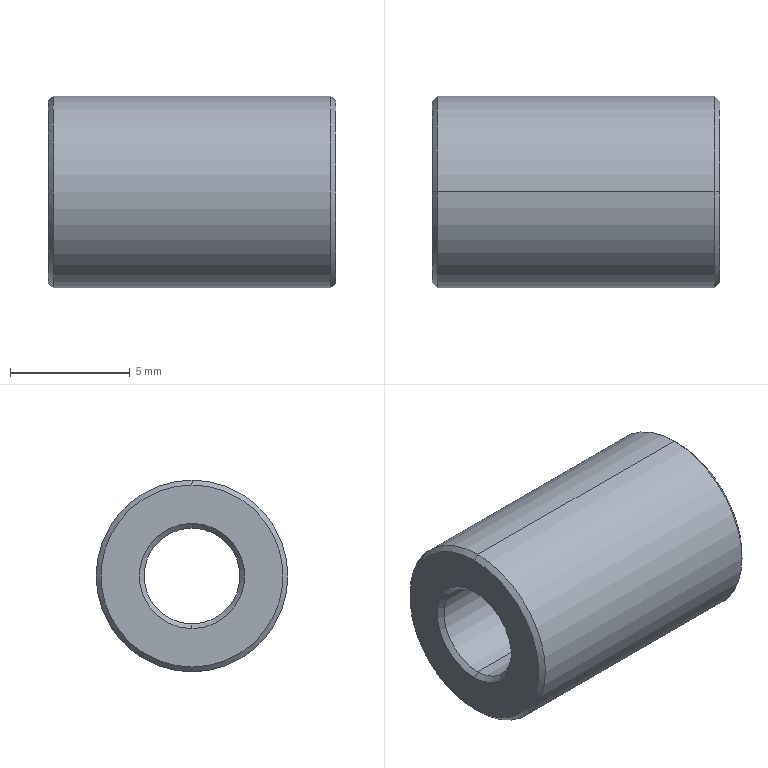Part | SolidWorks | features RefAxis 3, 3DProfileFeature 1, Chamfer 1, Revolution 1 | 1 solid | 14 faces | box 12 x 8 x 8 mm | volume 450.881 mm3 | cone 8 | cylinder 4 | plane 2 | commonest cylinder face diameters 4 x2 8 x2
STEP:
#1=CARTESIAN_POINT('',(0.,0.,3.8));
#2=VERTEX_POINT('',#1);
#3=CARTESIAN_POINT('',(0.,0.,-3.8));
#4=VERTEX_POINT('',#3);
#5=CARTESIAN_POINT('',(0.,0.,0.));
#6=DIRECTION('',(-1.,0.,0.));
#7=DIRECTION('',(0.,0.,-1.));
#8=AXIS2_PLACEMENT_3D('',#5,#6,#7);
#9=CIRCLE('',#8,3.8);
#10=EDGE_CURVE('',#2,#4,#9,.T.);
#11=ORIENTED_EDGE('',*,*,#10,.F.);
#12=CARTESIAN_POINT('',(0.2,0.,4.));
#13=VERTEX_POINT('',#12);
#14=CARTESIAN_POINT('',(0.,0.,3.8));
#15=DIRECTION('',(0.7071,0.,0.7071));
#16=VECTOR('',#15,1000.);
#17=LINE('',#14,#16);
#18=EDGE_CURVE('',#2,#13,#17,.T.);
#19=ORIENTED_EDGE('',*,*,#18,.T.);
#20=CARTESIAN_POINT('',(0.2,0.,-4.));
#21=VERTEX_POINT('',#20);
#22=CARTESIAN_POINT('',(0.2,0.,0.));
#23=DIRECTION('',(1.,0.,0.));
#24=DIRECTION('',(0.,0.,-1.));
#25=AXIS2_PLACEMENT_3D('',#22,#23,#24);
#26=CIRCLE('',#25,4.);
#27=EDGE_CURVE('',#21,#13,#26,.T.);
#28=ORIENTED_EDGE('',*,*,#27,.F.);
#29=CARTESIAN_POINT('',(0.,0.,-3.8));
#30=DIRECTION('',(0.7071,0.,-0.7071));
#31=VECTOR('',#30,1000.);
#32=LINE('',#29,#31);
#33=EDGE_CURVE('',#4,#21,#32,.T.);
#34=ORIENTED_EDGE('',*,*,#33,.F.);
#35=EDGE_LOOP('',(#11,#19,#28,#34));
#36=FACE_OUTER_BOUND('',#35,.T.);
#37=CARTESIAN_POINT('',(0.,0.,0.));
#38=DIRECTION('',(1.,0.,0.));
#39=DIRECTION('',(0.,0.,-1.));
#40=AXIS2_PLACEMENT_3D('',#37,#38,#39);
#41=CONICAL_SURFACE('',#40,3.8,0.7854);
#42=ADVANCED_FACE('',(#36),#41,.T.);
#43=CARTESIAN_POINT('',(12.,0.,-3.8));
#44=VERTEX_POINT('',#43);
#45=CARTESIAN_POINT('',(12.,0.,3.8));
#46=VERTEX_POINT('',#45);
#47=CARTESIAN_POINT('',(12.,0.,0.));
#48=DIRECTION('',(1.,0.,0.));
#49=DIRECTION('',(0.,0.,1.));
#50=AXIS2_PLACEMENT_3D('',#47,#48,#49);
#51=CIRCLE('',#50,3.8);
#52=EDGE_CURVE('',#44,#46,#51,.T.);
#53=ORIENTED_EDGE('',*,*,#52,.F.);
#54=CARTESIAN_POINT('',(11.8,0.,-4.));
#55=VERTEX_POINT('',#54);
#56=CARTESIAN_POINT('',(11.8,0.,-4.));
#57=DIRECTION('',(-0.7071,0.,-0.7071));
#58=VECTOR('',#57,1000.);
#59=LINE('',#56,#58);
#60=EDGE_CURVE('',#44,#55,#59,.T.);
#61=ORIENTED_EDGE('',*,*,#60,.T.);
#62=CARTESIAN_POINT('',(11.8,0.,4.));
#63=VERTEX_POINT('',#62);
#64=CARTESIAN_POINT('',(11.8,0.,0.));
#65=DIRECTION('',(-1.,0.,0.));
#66=DIRECTION('',(0.,0.,1.));
#67=AXIS2_PLACEMENT_3D('',#64,#65,#66);
#68=CIRCLE('',#67,4.);
#69=EDGE_CURVE('',#63,#55,#68,.T.);
#70=ORIENTED_EDGE('',*,*,#69,.F.);
#71=CARTESIAN_POINT('',(11.8,0.,4.));
#72=DIRECTION('',(-0.7071,0.,0.7071));
#73=VECTOR('',#72,1000.);
#74=LINE('',#71,#73);
#75=EDGE_CURVE('',#46,#63,#74,.T.);
#76=ORIENTED_EDGE('',*,*,#75,.F.);
#77=EDGE_LOOP('',(#53,#61,#70,#76));
#78=FACE_OUTER_BOUND('',#77,.T.);
#79=CARTESIAN_POINT('',(11.8,0.,0.));
#80=DIRECTION('',(-1.,0.,0.));
#81=DIRECTION('',(0.,0.,1.));
#82=AXIS2_PLACEMENT_3D('',#79,#80,#81);
#83=CONICAL_SURFACE('',#82,4.,0.7854);
#84=ADVANCED_FACE('',(#78),#83,.T.);
#85=CARTESIAN_POINT('',(0.2,0.,-2.));
#86=VERTEX_POINT('',#85);
#87=CARTESIAN_POINT('',(0.2,0.,2.));
#88=VERTEX_POINT('',#87);
#89=CARTESIAN_POINT('',(0.2,0.,0.));
#90=DIRECTION('',(-1.,0.,0.));
#91=DIRECTION('',(0.,0.,-1.));
#92=AXIS2_PLACEMENT_3D('',#89,#90,#91);
#93=CIRCLE('',#92,2.);
#94=EDGE_CURVE('',#86,#88,#93,.T.);
#95=ORIENTED_EDGE('',*,*,#94,.F.);
#96=CARTESIAN_POINT('',(0.,0.,-2.2));
#97=VERTEX_POINT('',#96);
#98=CARTESIAN_POINT('',(0.2,0.,-2.));
#99=DIRECTION('',(-0.7071,0.,-0.7071));
#100=VECTOR('',#99,1000.);
#101=LINE('',#98,#100);
#102=EDGE_CURVE('',#86,#97,#101,.T.);
#103=ORIENTED_EDGE('',*,*,#102,.T.);
#104=CARTESIAN_POINT('',(0.,0.,2.2));
#105=VERTEX_POINT('',#104);
#106=CARTESIAN_POINT('',(0.,0.,0.));
#107=DIRECTION('',(1.,0.,0.));
#108=DIRECTION('',(0.,0.,-1.));
#109=AXIS2_PLACEMENT_3D('',#106,#107,#108);
#110=CIRCLE('',#109,2.2);
#111=EDGE_CURVE('',#105,#97,#110,.T.);
#112=ORIENTED_EDGE('',*,*,#111,.F.);
#113=CARTESIAN_POINT('',(0.2,0.,2.));
#114=DIRECTION('',(-0.7071,0.,0.7071));
#115=VECTOR('',#114,1000.);
#116=LINE('',#113,#115);
#117=EDGE_CURVE('',#88,#105,#116,.T.);
#118=ORIENTED_EDGE('',*,*,#117,.F.);
#119=EDGE_LOOP('',(#95,#103,#112,#118));
#120=FACE_OUTER_BOUND('',#119,.T.);
#121=CARTESIAN_POINT('',(0.2,0.,0.));
#122=DIRECTION('',(-1.,0.,0.));
#123=DIRECTION('',(0.,0.,1.));
#124=AXIS2_PLACEMENT_3D('',#121,#122,#123);
#125=CONICAL_SURFACE('',#124,2.,0.7854);
#126=ADVANCED_FACE('',(#120),#125,.F.);
#127=CARTESIAN_POINT('',(11.8,0.,2.));
#128=VERTEX_POINT('',#127);
#129=CARTESIAN_POINT('',(11.8,0.,-2.));
#130=VERTEX_POINT('',#129);
#131=CARTESIAN_POINT('',(11.8,0.,0.));
#132=DIRECTION('',(1.,0.,0.));
#133=DIRECTION('',(0.,0.,1.));
#134=AXIS2_PLACEMENT_3D('',#131,#132,#133);
#135=CIRCLE('',#134,2.);
#136=EDGE_CURVE('',#128,#130,#135,.T.);
#137=ORIENTED_EDGE('',*,*,#136,.F.);
#138=CARTESIAN_POINT('',(12.,0.,2.2));
#139=VERTEX_POINT('',#138);
#140=CARTESIAN_POINT('',(12.,0.,2.2));
#141=DIRECTION('',(0.7071,0.,0.7071));
#142=VECTOR('',#141,1000.);
#143=LINE('',#140,#142);
#144=EDGE_CURVE('',#128,#139,#143,.T.);
#145=ORIENTED_EDGE('',*,*,#144,.T.);
#146=CARTESIAN_POINT('',(12.,0.,-2.2));
#147=VERTEX_POINT('',#146);
#148=CARTESIAN_POINT('',(12.,0.,0.));
#149=DIRECTION('',(-1.,0.,0.));
#150=DIRECTION('',(0.,0.,1.));
#151=AXIS2_PLACEMENT_3D('',#148,#149,#150);
#152=CIRCLE('',#151,2.2);
#153=EDGE_CURVE('',#147,#139,#152,.T.);
#154=ORIENTED_EDGE('',*,*,#153,.F.);
#155=CARTESIAN_POINT('',(12.,0.,-2.2));
#156=DIRECTION('',(0.7071,0.,-0.7071));
#157=VECTOR('',#156,1000.);
#158=LINE('',#155,#157);
#159=EDGE_CURVE('',#130,#147,#158,.T.);
#160=ORIENTED_EDGE('',*,*,#159,.F.);
#161=EDGE_LOOP('',(#137,#145,#154,#160));
#162=FACE_OUTER_BOUND('',#161,.T.);
#163=CARTESIAN_POINT('',(12.,0.,0.));
#164=DIRECTION('',(1.,0.,0.));
#165=DIRECTION('',(0.,0.,-1.));
#166=AXIS2_PLACEMENT_3D('',#163,#164,#165);
#167=CONICAL_SURFACE('',#166,2.2,0.7854);
#168=ADVANCED_FACE('',(#162),#167,.F.);
#169=ORIENTED_EDGE('',*,*,#69,.T.);
#170=CARTESIAN_POINT('',(12.,0.,-4.));
#171=DIRECTION('',(-1.,0.,0.));
#172=VECTOR('',#171,1000.);
#173=LINE('',#170,#172);
#174=EDGE_CURVE('',#55,#21,#173,.T.);
#175=ORIENTED_EDGE('',*,*,#174,.T.);
#176=ORIENTED_EDGE('',*,*,#27,.T.);
#177=CARTESIAN_POINT('',(12.,0.,4.));
#178=DIRECTION('',(-1.,0.,0.));
#179=VECTOR('',#178,1000.);
#180=LINE('',#177,#179);
#181=EDGE_CURVE('',#63,#13,#180,.T.);
#182=ORIENTED_EDGE('',*,*,#181,.F.);
#183=EDGE_LOOP('',(#169,#175,#176,#182));
#184=FACE_OUTER_BOUND('',#183,.T.);
#185=CARTESIAN_POINT('',(12.,0.,0.));
#186=DIRECTION('',(-1.,0.,0.));
#187=DIRECTION('',(0.,0.,1.));
#188=AXIS2_PLACEMENT_3D('',#185,#186,#187);
#189=CYLINDRICAL_SURFACE('',#188,4.);
#190=ADVANCED_FACE('',(#184),#189,.T.);
#191=ORIENTED_EDGE('',*,*,#136,.T.);
#192=CARTESIAN_POINT('',(12.,0.,-2.));
#193=DIRECTION('',(-1.,0.,0.));
#194=VECTOR('',#193,1000.);
#195=LINE('',#192,#194);
#196=EDGE_CURVE('',#130,#86,#195,.T.);
#197=ORIENTED_EDGE('',*,*,#196,.T.);
#198=ORIENTED_EDGE('',*,*,#94,.T.);
#199=CARTESIAN_POINT('',(12.,0.,2.));
#200=DIRECTION('',(-1.,0.,0.));
#201=VECTOR('',#200,1000.);
#202=LINE('',#199,#201);
#203=EDGE_CURVE('',#128,#88,#202,.T.);
#204=ORIENTED_EDGE('',*,*,#203,.F.);
#205=EDGE_LOOP('',(#191,#197,#198,#204));
#206=FACE_OUTER_BOUND('',#205,.T.);
#207=CARTESIAN_POINT('',(12.,0.,0.));
#208=DIRECTION('',(-1.,0.,0.));
#209=DIRECTION('',(0.,0.,1.));
#210=AXIS2_PLACEMENT_3D('',#207,#208,#209);
#211=CYLINDRICAL_SURFACE('',#210,2.);
#212=ADVANCED_FACE('',(#206),#211,.F.);
#213=ORIENTED_EDGE('',*,*,#111,.T.);
#214=CARTESIAN_POINT('',(0.,0.,0.));
#215=DIRECTION('',(1.,0.,0.));
#216=DIRECTION('',(0.,0.,-1.));
#217=AXIS2_PLACEMENT_3D('',#214,#215,#216);
#218=CIRCLE('',#217,2.2);
#219=EDGE_CURVE('',#97,#105,#218,.T.);
#220=ORIENTED_EDGE('',*,*,#219,.T.);
#221=EDGE_LOOP('',(#213,#220));
#222=FACE_BOUND('',#221,.T.);
#223=CARTESIAN_POINT('',(0.,0.,0.));
#224=DIRECTION('',(-1.,0.,0.));
#225=DIRECTION('',(0.,0.,-1.));
#226=AXIS2_PLACEMENT_3D('',#223,#224,#225);
#227=CIRCLE('',#226,3.8);
#228=EDGE_CURVE('',#4,#2,#227,.T.);
#229=ORIENTED_EDGE('',*,*,#228,.T.);
#230=ORIENTED_EDGE('',*,*,#10,.T.);
#231=EDGE_LOOP('',(#229,#230));
#232=FACE_OUTER_BOUND('',#231,.T.);
#233=CARTESIAN_POINT('',(0.,3.7,0.));
#234=DIRECTION('',(1.,0.,0.));
#235=DIRECTION('',(0.,0.,-1.));
#236=AXIS2_PLACEMENT_3D('',#233,#234,#235);
#237=PLANE('',#236);
#238=ADVANCED_FACE('',(#222,#232),#237,.F.);
#239=ORIENTED_EDGE('',*,*,#196,.F.);
#240=CARTESIAN_POINT('',(11.8,0.,0.));
#241=DIRECTION('',(1.,0.,0.));
#242=DIRECTION('',(0.,0.,1.));
#243=AXIS2_PLACEMENT_3D('',#240,#241,#242);
#244=CIRCLE('',#243,2.);
#245=EDGE_CURVE('',#130,#128,#244,.T.);
#246=ORIENTED_EDGE('',*,*,#245,.T.);
#247=ORIENTED_EDGE('',*,*,#203,.T.);
#248=CARTESIAN_POINT('',(0.2,0.,0.));
#249=DIRECTION('',(-1.,0.,0.));
#250=DIRECTION('',(0.,0.,-1.));
#251=AXIS2_PLACEMENT_3D('',#248,#249,#250);
#252=CIRCLE('',#251,2.);
#253=EDGE_CURVE('',#88,#86,#252,.T.);
#254=ORIENTED_EDGE('',*,*,#253,.T.);
#255=EDGE_LOOP('',(#239,#246,#247,#254));
#256=FACE_OUTER_BOUND('',#255,.T.);
#257=CARTESIAN_POINT('',(12.,0.,0.));
#258=DIRECTION('',(-1.,0.,0.));
#259=DIRECTION('',(0.,0.,1.));
#260=AXIS2_PLACEMENT_3D('',#257,#258,#259);
#261=CYLINDRICAL_SURFACE('',#260,2.);
#262=ADVANCED_FACE('',(#256),#261,.F.);
#263=ORIENTED_EDGE('',*,*,#153,.T.);
#264=CARTESIAN_POINT('',(12.,0.,0.));
#265=DIRECTION('',(-1.,0.,0.));
#266=DIRECTION('',(0.,0.,1.));
#267=AXIS2_PLACEMENT_3D('',#264,#265,#266);
#268=CIRCLE('',#267,2.2);
#269=EDGE_CURVE('',#139,#147,#268,.T.);
#270=ORIENTED_EDGE('',*,*,#269,.T.);
#271=EDGE_LOOP('',(#263,#270));
#272=FACE_BOUND('',#271,.T.);
#273=CARTESIAN_POINT('',(12.,0.,0.));
#274=DIRECTION('',(1.,0.,0.));
#275=DIRECTION('',(0.,0.,1.));
#276=AXIS2_PLACEMENT_3D('',#273,#274,#275);
#277=CIRCLE('',#276,3.8);
#278=EDGE_CURVE('',#46,#44,#277,.T.);
#279=ORIENTED_EDGE('',*,*,#278,.T.);
#280=ORIENTED_EDGE('',*,*,#52,.T.);
#281=EDGE_LOOP('',(#279,#280));
#282=FACE_OUTER_BOUND('',#281,.T.);
#283=CARTESIAN_POINT('',(12.,3.7,0.));
#284=DIRECTION('',(-1.,0.,0.));
#285=DIRECTION('',(0.,0.,1.));
#286=AXIS2_PLACEMENT_3D('',#283,#284,#285);
#287=PLANE('',#286);
#288=ADVANCED_FACE('',(#272,#282),#287,.F.);
#289=ORIENTED_EDGE('',*,*,#174,.F.);
#290=CARTESIAN_POINT('',(11.8,0.,0.));
#291=DIRECTION('',(-1.,0.,0.));
#292=DIRECTION('',(0.,0.,1.));
#293=AXIS2_PLACEMENT_3D('',#290,#291,#292);
#294=CIRCLE('',#293,4.);
#295=EDGE_CURVE('',#55,#63,#294,.T.);
#296=ORIENTED_EDGE('',*,*,#295,.T.);
#297=ORIENTED_EDGE('',*,*,#181,.T.);
#298=CARTESIAN_POINT('',(0.2,0.,0.));
#299=DIRECTION('',(1.,0.,0.));
#300=DIRECTION('',(0.,0.,-1.));
#301=AXIS2_PLACEMENT_3D('',#298,#299,#300);
#302=CIRCLE('',#301,4.);
#303=EDGE_CURVE('',#13,#21,#302,.T.);
#304=ORIENTED_EDGE('',*,*,#303,.T.);
#305=EDGE_LOOP('',(#289,#296,#297,#304));
#306=FACE_OUTER_BOUND('',#305,.T.);
#307=CARTESIAN_POINT('',(12.,0.,0.));
#308=DIRECTION('',(-1.,0.,0.));
#309=DIRECTION('',(0.,0.,1.));
#310=AXIS2_PLACEMENT_3D('',#307,#308,#309);
#311=CYLINDRICAL_SURFACE('',#310,4.);
#312=ADVANCED_FACE('',(#306),#311,.T.);
#313=ORIENTED_EDGE('',*,*,#144,.F.);
#314=ORIENTED_EDGE('',*,*,#245,.F.);
#315=ORIENTED_EDGE('',*,*,#159,.T.);
#316=ORIENTED_EDGE('',*,*,#269,.F.);
#317=EDGE_LOOP('',(#313,#314,#315,#316));
#318=FACE_OUTER_BOUND('',#317,.T.);
#319=CARTESIAN_POINT('',(12.,0.,0.));
#320=DIRECTION('',(1.,0.,0.));
#321=DIRECTION('',(0.,0.,-1.));
#322=AXIS2_PLACEMENT_3D('',#319,#320,#321);
#323=CONICAL_SURFACE('',#322,2.2,0.7854);
#324=ADVANCED_FACE('',(#318),#323,.F.);
#325=ORIENTED_EDGE('',*,*,#102,.F.);
#326=ORIENTED_EDGE('',*,*,#253,.F.);
#327=ORIENTED_EDGE('',*,*,#117,.T.);
#328=ORIENTED_EDGE('',*,*,#219,.F.);
#329=EDGE_LOOP('',(#325,#326,#327,#328));
#330=FACE_OUTER_BOUND('',#329,.T.);
#331=CARTESIAN_POINT('',(0.2,0.,0.));
#332=DIRECTION('',(-1.,0.,0.));
#333=DIRECTION('',(0.,0.,1.));
#334=AXIS2_PLACEMENT_3D('',#331,#332,#333);
#335=CONICAL_SURFACE('',#334,2.,0.7854);
#336=ADVANCED_FACE('',(#330),#335,.F.);
#337=ORIENTED_EDGE('',*,*,#60,.F.);
#338=ORIENTED_EDGE('',*,*,#278,.F.);
#339=ORIENTED_EDGE('',*,*,#75,.T.);
#340=ORIENTED_EDGE('',*,*,#295,.F.);
#341=EDGE_LOOP('',(#337,#338,#339,#340));
#342=FACE_OUTER_BOUND('',#341,.T.);
#343=CARTESIAN_POINT('',(11.8,0.,0.));
#344=DIRECTION('',(-1.,0.,0.));
#345=DIRECTION('',(0.,0.,1.));
#346=AXIS2_PLACEMENT_3D('',#343,#344,#345);
#347=CONICAL_SURFACE('',#346,4.,0.7854);
#348=ADVANCED_FACE('',(#342),#347,.T.);
#349=ORIENTED_EDGE('',*,*,#18,.F.);
#350=ORIENTED_EDGE('',*,*,#228,.F.);
#351=ORIENTED_EDGE('',*,*,#33,.T.);
#352=ORIENTED_EDGE('',*,*,#303,.F.);
#353=EDGE_LOOP('',(#349,#350,#351,#352));
#354=FACE_OUTER_BOUND('',#353,.T.);
#355=CARTESIAN_POINT('',(0.,0.,0.));
#356=DIRECTION('',(1.,0.,0.));
#357=DIRECTION('',(0.,0.,-1.));
#358=AXIS2_PLACEMENT_3D('',#355,#356,#357);
#359=CONICAL_SURFACE('',#358,3.8,0.7854);
#360=ADVANCED_FACE('',(#354),#359,.T.);
#361=CLOSED_SHELL('',(#42,#84,#126,#168,#190,#212,#238,#262,#288,#312,#324,#336,#348,#360));
#362=MANIFOLD_SOLID_BREP('',#361);
#363=CARTESIAN_POINT('',(0.,0.,0.));
#364=DIRECTION('',(0.,0.,1.));
#365=DIRECTION('',(1.,0.,0.));
#366=AXIS2_PLACEMENT_3D('',#363,#364,#365);
#367=(LENGTH_UNIT()NAMED_UNIT(*)SI_UNIT(.MILLI.,.METRE.));
#368=UNCERTAINTY_MEASURE_WITH_UNIT(LENGTH_MEASURE(0.00001),#367,'','');
#369=(NAMED_UNIT(*)PLANE_ANGLE_UNIT()SI_UNIT($,.RADIAN.));
#370=(NAMED_UNIT(*)SI_UNIT($,.STERADIAN.)SOLID_ANGLE_UNIT());
#371=(GEOMETRIC_REPRESENTATION_CONTEXT(3)GLOBAL_UNCERTAINTY_ASSIGNED_CONTEXT((#368))GLOBAL_UNIT_ASSIGNED_CONTEXT((#367,#369,#370))REPRESENTATION_CONTEXT('',''));
#372=ADVANCED_BREP_SHAPE_REPRESENTATION('',(#362,#366),#371);